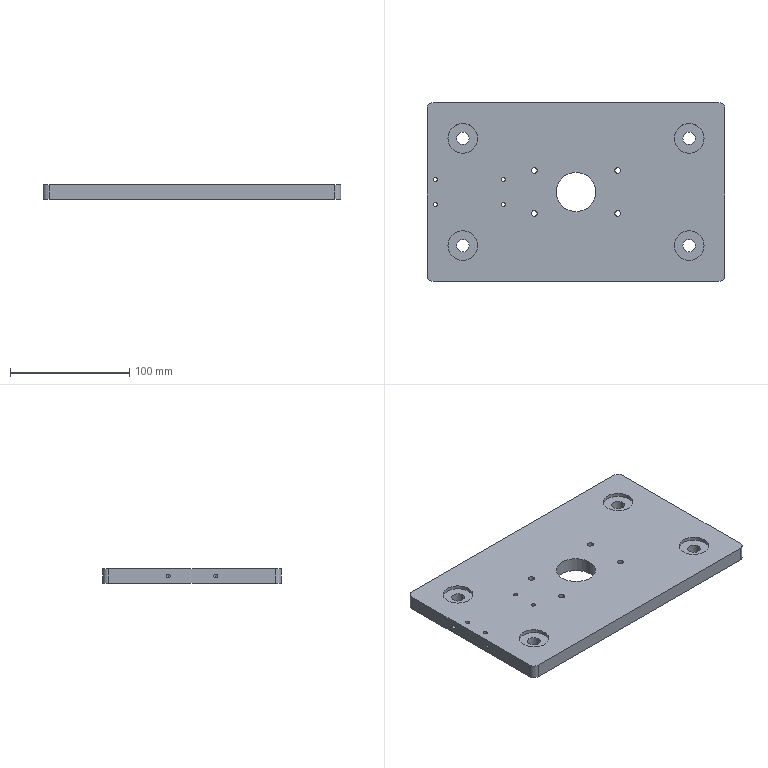Part | STEP file | 03-29 press fixed plate | 1 solid | 64 faces | box 250 x 150 x 12 mm | volume 428713 mm3 | cylinder 46 | plane 10 | cone 8 | commonest cylinder face diameters 3.3 x16 5 x8 10.5 x8 25 x8 10 x4 33 x2